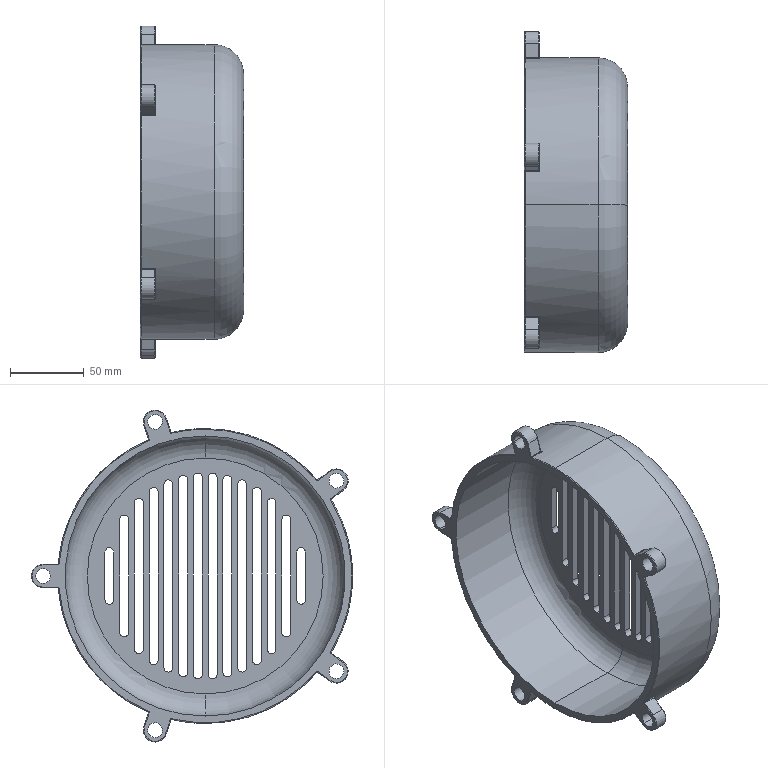Part | SolidWorks | 1 solid | 200 faces | box 70 x 218 x 225.232 mm | volume 296939 mm3 | cylinder 83 | plane 56 | torus 34 | spline 20 | cone 7 | commonest cylinder face diameters 6 x42 1 x22 10 x10 16 x5 190 x2 200 x2